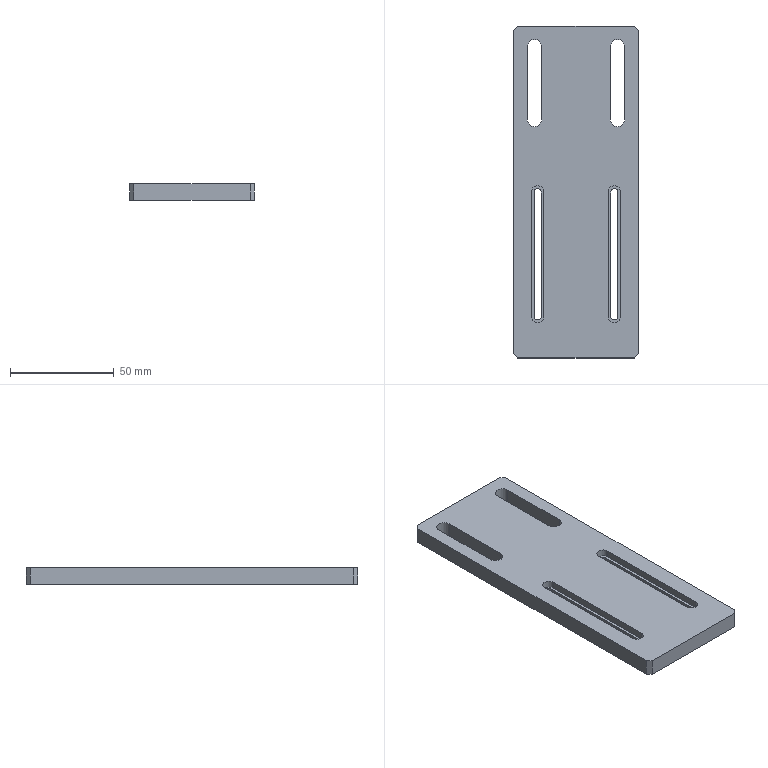Part | NX | 1 solid | 36 faces | box 60 x 160 x 8 mm | volume 67600 mm3 | plane 24 | cylinder 12 | commonest cylinder face diameters 3.4 x4 6 x4 7 x4
STEP:
#1=CARTESIAN_POINT('',(16.8,0.,4.6));
#2=VERTEX_POINT('',#1);
#3=CARTESIAN_POINT('',(20.2,0.,4.6));
#4=VERTEX_POINT('',#3);
#5=CARTESIAN_POINT('',(18.5,0.,4.6));
#6=DIRECTION('',(0.,0.,1.));
#7=DIRECTION('',(1.,0.,0.));
#8=AXIS2_PLACEMENT_3D('',#5,#6,#7);
#9=CIRCLE('',#8,1.7);
#10=EDGE_CURVE('',#2,#4,#9,.F.);
#11=ORIENTED_EDGE('',*,*,#10,.F.);
#12=CARTESIAN_POINT('',(16.8,0.,0.));
#13=VERTEX_POINT('',#12);
#14=CARTESIAN_POINT('',(16.8,0.,0.));
#15=DIRECTION('',(0.,0.,1.));
#16=VECTOR('',#15,1000.);
#17=LINE('',#14,#16);
#18=EDGE_CURVE('',#13,#2,#17,.T.);
#19=ORIENTED_EDGE('',*,*,#18,.F.);
#20=CARTESIAN_POINT('',(20.2,0.,0.));
#21=VERTEX_POINT('',#20);
#22=CARTESIAN_POINT('',(18.5,0.,0.));
#23=DIRECTION('',(0.,0.,1.));
#24=DIRECTION('',(1.,0.,0.));
#25=AXIS2_PLACEMENT_3D('',#22,#23,#24);
#26=CIRCLE('',#25,1.7);
#27=EDGE_CURVE('',#21,#13,#26,.T.);
#28=ORIENTED_EDGE('',*,*,#27,.F.);
#29=CARTESIAN_POINT('',(20.2,0.,0.));
#30=DIRECTION('',(0.,0.,1.));
#31=VECTOR('',#30,1000.);
#32=LINE('',#29,#31);
#33=EDGE_CURVE('',#21,#4,#32,.T.);
#34=ORIENTED_EDGE('',*,*,#33,.T.);
#35=EDGE_LOOP('',(#11,#19,#28,#34));
#36=FACE_BOUND('',#35,.T.);
#37=CARTESIAN_POINT('',(18.5,0.,0.));
#38=DIRECTION('',(0.,0.,1.));
#39=DIRECTION('',(1.,0.,0.));
#40=AXIS2_PLACEMENT_3D('',#37,#38,#39);
#41=CYLINDRICAL_SURFACE('',#40,1.7);
#42=ADVANCED_FACE('',(#36),#41,.F.);
#43=CARTESIAN_POINT('',(20.2,-60.,4.6));
#44=VERTEX_POINT('',#43);
#45=CARTESIAN_POINT('',(20.2,0.,4.6));
#46=DIRECTION('',(0.,-1.,0.));
#47=VECTOR('',#46,1000.);
#48=LINE('',#45,#47);
#49=EDGE_CURVE('',#4,#44,#48,.T.);
#50=ORIENTED_EDGE('',*,*,#49,.F.);
#51=ORIENTED_EDGE('',*,*,#33,.F.);
#52=CARTESIAN_POINT('',(20.2,-60.,0.));
#53=VERTEX_POINT('',#52);
#54=CARTESIAN_POINT('',(20.2,0.,0.));
#55=DIRECTION('',(0.,1.,0.));
#56=VECTOR('',#55,1000.);
#57=LINE('',#54,#56);
#58=EDGE_CURVE('',#53,#21,#57,.T.);
#59=ORIENTED_EDGE('',*,*,#58,.F.);
#60=CARTESIAN_POINT('',(20.2,-60.,0.));
#61=DIRECTION('',(0.,0.,1.));
#62=VECTOR('',#61,1000.);
#63=LINE('',#60,#62);
#64=EDGE_CURVE('',#53,#44,#63,.T.);
#65=ORIENTED_EDGE('',*,*,#64,.T.);
#66=EDGE_LOOP('',(#50,#51,#59,#65));
#67=FACE_BOUND('',#66,.T.);
#68=CARTESIAN_POINT('',(20.2,0.,0.));
#69=DIRECTION('',(1.,0.,0.));
#70=DIRECTION('',(0.,1.,0.));
#71=AXIS2_PLACEMENT_3D('',#68,#69,#70);
#72=PLANE('',#71);
#73=ADVANCED_FACE('',(#67),#72,.F.);
#74=CARTESIAN_POINT('',(16.8,-60.,4.6));
#75=VERTEX_POINT('',#74);
#76=CARTESIAN_POINT('',(18.5,-60.,4.6));
#77=DIRECTION('',(0.,0.,1.));
#78=DIRECTION('',(1.,0.,0.));
#79=AXIS2_PLACEMENT_3D('',#76,#77,#78);
#80=CIRCLE('',#79,1.7);
#81=EDGE_CURVE('',#44,#75,#80,.F.);
#82=ORIENTED_EDGE('',*,*,#81,.F.);
#83=ORIENTED_EDGE('',*,*,#64,.F.);
#84=CARTESIAN_POINT('',(16.8,-60.,0.));
#85=VERTEX_POINT('',#84);
#86=CARTESIAN_POINT('',(18.5,-60.,0.));
#87=DIRECTION('',(0.,0.,1.));
#88=DIRECTION('',(1.,0.,0.));
#89=AXIS2_PLACEMENT_3D('',#86,#87,#88);
#90=CIRCLE('',#89,1.7);
#91=EDGE_CURVE('',#85,#53,#90,.T.);
#92=ORIENTED_EDGE('',*,*,#91,.F.);
#93=CARTESIAN_POINT('',(16.8,-60.,0.));
#94=DIRECTION('',(0.,0.,1.));
#95=VECTOR('',#94,1000.);
#96=LINE('',#93,#95);
#97=EDGE_CURVE('',#85,#75,#96,.T.);
#98=ORIENTED_EDGE('',*,*,#97,.T.);
#99=EDGE_LOOP('',(#82,#83,#92,#98));
#100=FACE_BOUND('',#99,.T.);
#101=CARTESIAN_POINT('',(18.5,-60.,0.));
#102=DIRECTION('',(0.,0.,1.));
#103=DIRECTION('',(1.,0.,0.));
#104=AXIS2_PLACEMENT_3D('',#101,#102,#103);
#105=CYLINDRICAL_SURFACE('',#104,1.7);
#106=ADVANCED_FACE('',(#100),#105,.F.);
#107=CARTESIAN_POINT('',(16.8,0.,4.6));
#108=DIRECTION('',(0.,1.,0.));
#109=VECTOR('',#108,1000.);
#110=LINE('',#107,#109);
#111=EDGE_CURVE('',#75,#2,#110,.T.);
#112=ORIENTED_EDGE('',*,*,#111,.F.);
#113=ORIENTED_EDGE('',*,*,#97,.F.);
#114=CARTESIAN_POINT('',(16.8,0.,0.));
#115=DIRECTION('',(0.,-1.,0.));
#116=VECTOR('',#115,1000.);
#117=LINE('',#114,#116);
#118=EDGE_CURVE('',#13,#85,#117,.T.);
#119=ORIENTED_EDGE('',*,*,#118,.F.);
#120=ORIENTED_EDGE('',*,*,#18,.T.);
#121=EDGE_LOOP('',(#112,#113,#119,#120));
#122=FACE_BOUND('',#121,.T.);
#123=CARTESIAN_POINT('',(16.8,0.,0.));
#124=DIRECTION('',(-1.,0.,0.));
#125=DIRECTION('',(0.,-1.,0.));
#126=AXIS2_PLACEMENT_3D('',#123,#124,#125);
#127=PLANE('',#126);
#128=ADVANCED_FACE('',(#122),#127,.F.);
#129=CARTESIAN_POINT('',(-20.2,0.,4.6));
#130=VERTEX_POINT('',#129);
#131=CARTESIAN_POINT('',(-16.8,0.,4.6));
#132=VERTEX_POINT('',#131);
#133=CARTESIAN_POINT('',(-18.5,0.,4.6));
#134=DIRECTION('',(0.,0.,1.));
#135=DIRECTION('',(1.,0.,0.));
#136=AXIS2_PLACEMENT_3D('',#133,#134,#135);
#137=CIRCLE('',#136,1.7);
#138=EDGE_CURVE('',#130,#132,#137,.F.);
#139=ORIENTED_EDGE('',*,*,#138,.F.);
#140=CARTESIAN_POINT('',(-20.2,0.,0.));
#141=VERTEX_POINT('',#140);
#142=CARTESIAN_POINT('',(-20.2,0.,0.));
#143=DIRECTION('',(0.,0.,1.));
#144=VECTOR('',#143,1000.);
#145=LINE('',#142,#144);
#146=EDGE_CURVE('',#141,#130,#145,.T.);
#147=ORIENTED_EDGE('',*,*,#146,.F.);
#148=CARTESIAN_POINT('',(-16.8,0.,0.));
#149=VERTEX_POINT('',#148);
#150=CARTESIAN_POINT('',(-18.5,0.,0.));
#151=DIRECTION('',(0.,0.,1.));
#152=DIRECTION('',(1.,0.,0.));
#153=AXIS2_PLACEMENT_3D('',#150,#151,#152);
#154=CIRCLE('',#153,1.7);
#155=EDGE_CURVE('',#149,#141,#154,.T.);
#156=ORIENTED_EDGE('',*,*,#155,.F.);
#157=CARTESIAN_POINT('',(-16.8,0.,0.));
#158=DIRECTION('',(0.,0.,1.));
#159=VECTOR('',#158,1000.);
#160=LINE('',#157,#159);
#161=EDGE_CURVE('',#149,#132,#160,.T.);
#162=ORIENTED_EDGE('',*,*,#161,.T.);
#163=EDGE_LOOP('',(#139,#147,#156,#162));
#164=FACE_BOUND('',#163,.T.);
#165=CARTESIAN_POINT('',(-18.5,0.,0.));
#166=DIRECTION('',(0.,0.,1.));
#167=DIRECTION('',(1.,0.,0.));
#168=AXIS2_PLACEMENT_3D('',#165,#166,#167);
#169=CYLINDRICAL_SURFACE('',#168,1.7);
#170=ADVANCED_FACE('',(#164),#169,.F.);
#171=CARTESIAN_POINT('',(-16.8,-60.,4.6));
#172=VERTEX_POINT('',#171);
#173=CARTESIAN_POINT('',(-16.8,0.,4.6));
#174=DIRECTION('',(0.,-1.,0.));
#175=VECTOR('',#174,1000.);
#176=LINE('',#173,#175);
#177=EDGE_CURVE('',#132,#172,#176,.T.);
#178=ORIENTED_EDGE('',*,*,#177,.F.);
#179=ORIENTED_EDGE('',*,*,#161,.F.);
#180=CARTESIAN_POINT('',(-16.8,-60.,0.));
#181=VERTEX_POINT('',#180);
#182=CARTESIAN_POINT('',(-16.8,0.,0.));
#183=DIRECTION('',(0.,1.,0.));
#184=VECTOR('',#183,1000.);
#185=LINE('',#182,#184);
#186=EDGE_CURVE('',#181,#149,#185,.T.);
#187=ORIENTED_EDGE('',*,*,#186,.F.);
#188=CARTESIAN_POINT('',(-16.8,-60.,0.));
#189=DIRECTION('',(0.,0.,1.));
#190=VECTOR('',#189,1000.);
#191=LINE('',#188,#190);
#192=EDGE_CURVE('',#181,#172,#191,.T.);
#193=ORIENTED_EDGE('',*,*,#192,.T.);
#194=EDGE_LOOP('',(#178,#179,#187,#193));
#195=FACE_BOUND('',#194,.T.);
#196=CARTESIAN_POINT('',(-16.8,0.,0.));
#197=DIRECTION('',(1.,0.,0.));
#198=DIRECTION('',(0.,0.,-1.));
#199=AXIS2_PLACEMENT_3D('',#196,#197,#198);
#200=PLANE('',#199);
#201=ADVANCED_FACE('',(#195),#200,.F.);
#202=CARTESIAN_POINT('',(-20.2,-60.,4.6));
#203=VERTEX_POINT('',#202);
#204=CARTESIAN_POINT('',(-18.5,-60.,4.6));
#205=DIRECTION('',(0.,0.,1.));
#206=DIRECTION('',(1.,0.,0.));
#207=AXIS2_PLACEMENT_3D('',#204,#205,#206);
#208=CIRCLE('',#207,1.7);
#209=EDGE_CURVE('',#172,#203,#208,.F.);
#210=ORIENTED_EDGE('',*,*,#209,.F.);
#211=ORIENTED_EDGE('',*,*,#192,.F.);
#212=CARTESIAN_POINT('',(-20.2,-60.,0.));
#213=VERTEX_POINT('',#212);
#214=CARTESIAN_POINT('',(-18.5,-60.,0.));
#215=DIRECTION('',(0.,0.,1.));
#216=DIRECTION('',(1.,0.,0.));
#217=AXIS2_PLACEMENT_3D('',#214,#215,#216);
#218=CIRCLE('',#217,1.7);
#219=EDGE_CURVE('',#213,#181,#218,.T.);
#220=ORIENTED_EDGE('',*,*,#219,.F.);
#221=CARTESIAN_POINT('',(-20.2,-60.,0.));
#222=DIRECTION('',(0.,0.,1.));
#223=VECTOR('',#222,1000.);
#224=LINE('',#221,#223);
#225=EDGE_CURVE('',#213,#203,#224,.T.);
#226=ORIENTED_EDGE('',*,*,#225,.T.);
#227=EDGE_LOOP('',(#210,#211,#220,#226));
#228=FACE_BOUND('',#227,.T.);
#229=CARTESIAN_POINT('',(-18.5,-60.,0.));
#230=DIRECTION('',(0.,0.,1.));
#231=DIRECTION('',(1.,0.,0.));
#232=AXIS2_PLACEMENT_3D('',#229,#230,#231);
#233=CYLINDRICAL_SURFACE('',#232,1.7);
#234=ADVANCED_FACE('',(#228),#233,.F.);
#235=CARTESIAN_POINT('',(-20.2,0.,4.6));
#236=DIRECTION('',(0.,1.,0.));
#237=VECTOR('',#236,1000.);
#238=LINE('',#235,#237);
#239=EDGE_CURVE('',#203,#130,#238,.T.);
#240=ORIENTED_EDGE('',*,*,#239,.F.);
#241=ORIENTED_EDGE('',*,*,#225,.F.);
#242=CARTESIAN_POINT('',(-20.2,0.,0.));
#243=DIRECTION('',(0.,-1.,0.));
#244=VECTOR('',#243,1000.);
#245=LINE('',#242,#244);
#246=EDGE_CURVE('',#141,#213,#245,.T.);
#247=ORIENTED_EDGE('',*,*,#246,.F.);
#248=ORIENTED_EDGE('',*,*,#146,.T.);
#249=EDGE_LOOP('',(#240,#241,#247,#248));
#250=FACE_BOUND('',#249,.T.);
#251=CARTESIAN_POINT('',(-20.2,0.,0.));
#252=DIRECTION('',(-1.,0.,0.));
#253=DIRECTION('',(0.,0.,1.));
#254=AXIS2_PLACEMENT_3D('',#251,#252,#253);
#255=PLANE('',#254);
#256=ADVANCED_FACE('',(#250),#255,.F.);
#257=CARTESIAN_POINT('',(-30.,78.,0.));
#258=VERTEX_POINT('',#257);
#259=CARTESIAN_POINT('',(-30.,-78.,0.));
#260=VERTEX_POINT('',#259);
#261=CARTESIAN_POINT('',(-30.,-80.,0.));
#262=DIRECTION('',(0.,-1.,0.));
#263=VECTOR('',#262,1000.);
#264=LINE('',#261,#263);
#265=EDGE_CURVE('',#258,#260,#264,.T.);
#266=ORIENTED_EDGE('',*,*,#265,.T.);
#267=CARTESIAN_POINT('',(-30.,-78.,8.));
#268=VERTEX_POINT('',#267);
#269=CARTESIAN_POINT('',(-30.,-78.,8.));
#270=DIRECTION('',(0.,0.,1.));
#271=VECTOR('',#270,1000.);
#272=LINE('',#269,#271);
#273=EDGE_CURVE('',#260,#268,#272,.T.);
#274=ORIENTED_EDGE('',*,*,#273,.T.);
#275=CARTESIAN_POINT('',(-30.,78.,8.));
#276=VERTEX_POINT('',#275);
#277=CARTESIAN_POINT('',(-30.,-80.,8.));
#278=DIRECTION('',(0.,-1.,0.));
#279=VECTOR('',#278,1000.);
#280=LINE('',#277,#279);
#281=EDGE_CURVE('',#276,#268,#280,.T.);
#282=ORIENTED_EDGE('',*,*,#281,.F.);
#283=CARTESIAN_POINT('',(-30.,78.,8.));
#284=DIRECTION('',(0.,0.,-1.));
#285=VECTOR('',#284,1000.);
#286=LINE('',#283,#285);
#287=EDGE_CURVE('',#276,#258,#286,.T.);
#288=ORIENTED_EDGE('',*,*,#287,.T.);
#289=EDGE_LOOP('',(#266,#274,#282,#288));
#290=FACE_BOUND('',#289,.T.);
#291=CARTESIAN_POINT('',(-30.,-80.,8.));
#292=DIRECTION('',(1.,0.,0.));
#293=DIRECTION('',(0.,0.,-1.));
#294=AXIS2_PLACEMENT_3D('',#291,#292,#293);
#295=PLANE('',#294);
#296=ADVANCED_FACE('',(#290),#295,.F.);
#297=CARTESIAN_POINT('',(-28.,-80.,0.));
#298=VERTEX_POINT('',#297);
#299=CARTESIAN_POINT('',(28.,-80.,0.));
#300=VERTEX_POINT('',#299);
#301=CARTESIAN_POINT('',(30.,-80.,0.));
#302=DIRECTION('',(1.,0.,0.));
#303=VECTOR('',#302,1000.);
#304=LINE('',#301,#303);
#305=EDGE_CURVE('',#298,#300,#304,.T.);
#306=ORIENTED_EDGE('',*,*,#305,.T.);
#307=CARTESIAN_POINT('',(28.,-80.,8.));
#308=VERTEX_POINT('',#307);
#309=CARTESIAN_POINT('',(28.,-80.,8.));
#310=DIRECTION('',(0.,0.,1.));
#311=VECTOR('',#310,1000.);
#312=LINE('',#309,#311);
#313=EDGE_CURVE('',#300,#308,#312,.T.);
#314=ORIENTED_EDGE('',*,*,#313,.T.);
#315=CARTESIAN_POINT('',(-28.,-80.,8.));
#316=VERTEX_POINT('',#315);
#317=CARTESIAN_POINT('',(30.,-80.,8.));
#318=DIRECTION('',(1.,0.,0.));
#319=VECTOR('',#318,1000.);
#320=LINE('',#317,#319);
#321=EDGE_CURVE('',#316,#308,#320,.T.);
#322=ORIENTED_EDGE('',*,*,#321,.F.);
#323=CARTESIAN_POINT('',(-28.,-80.,8.));
#324=DIRECTION('',(0.,0.,-1.));
#325=VECTOR('',#324,1000.);
#326=LINE('',#323,#325);
#327=EDGE_CURVE('',#316,#298,#326,.T.);
#328=ORIENTED_EDGE('',*,*,#327,.T.);
#329=EDGE_LOOP('',(#306,#314,#322,#328));
#330=FACE_BOUND('',#329,.T.);
#331=CARTESIAN_POINT('',(30.,-80.,8.));
#332=DIRECTION('',(0.,1.,0.));
#333=DIRECTION('',(-1.,0.,0.));
#334=AXIS2_PLACEMENT_3D('',#331,#332,#333);
#335=PLANE('',#334);
#336=ADVANCED_FACE('',(#330),#335,.F.);
#337=CARTESIAN_POINT('',(30.,-78.,8.));
#338=VERTEX_POINT('',#337);
#339=CARTESIAN_POINT('',(30.,78.,8.));
#340=VERTEX_POINT('',#339);
#341=CARTESIAN_POINT('',(30.,-80.,8.));
#342=DIRECTION('',(0.,1.,0.));
#343=VECTOR('',#342,1000.);
#344=LINE('',#341,#343);
#345=EDGE_CURVE('',#338,#340,#344,.T.);
#346=ORIENTED_EDGE('',*,*,#345,.F.);
#347=CARTESIAN_POINT('',(30.,-78.,0.));
#348=VERTEX_POINT('',#347);
#349=CARTESIAN_POINT('',(30.,-78.,8.));
#350=DIRECTION('',(0.,0.,-1.));
#351=VECTOR('',#350,1000.);
#352=LINE('',#349,#351);
#353=EDGE_CURVE('',#338,#348,#352,.T.);
#354=ORIENTED_EDGE('',*,*,#353,.T.);
#355=CARTESIAN_POINT('',(30.,78.,0.));
#356=VERTEX_POINT('',#355);
#357=CARTESIAN_POINT('',(30.,-80.,0.));
#358=DIRECTION('',(0.,1.,0.));
#359=VECTOR('',#358,1000.);
#360=LINE('',#357,#359);
#361=EDGE_CURVE('',#348,#356,#360,.T.);
#362=ORIENTED_EDGE('',*,*,#361,.T.);
#363=CARTESIAN_POINT('',(30.,78.,8.));
#364=DIRECTION('',(0.,0.,1.));
#365=VECTOR('',#364,1000.);
#366=LINE('',#363,#365);
#367=EDGE_CURVE('',#356,#340,#366,.T.);
#368=ORIENTED_EDGE('',*,*,#367,.T.);
#369=EDGE_LOOP('',(#346,#354,#362,#368));
#370=FACE_BOUND('',#369,.T.);
#371=CARTESIAN_POINT('',(30.,-80.,8.));
#372=DIRECTION('',(-1.,0.,0.));
#373=DIRECTION('',(0.,0.,1.));
#374=AXIS2_PLACEMENT_3D('',#371,#372,#373);
#375=PLANE('',#374);
#376=ADVANCED_FACE('',(#370),#375,.F.);
#377=CARTESIAN_POINT('',(28.,80.,0.));
#378=VERTEX_POINT('',#377);
#379=CARTESIAN_POINT('',(-28.,80.,0.));
#380=VERTEX_POINT('',#379);
#381=CARTESIAN_POINT('',(30.,80.,0.));
#382=DIRECTION('',(-1.,0.,0.));
#383=VECTOR('',#382,1000.);
#384=LINE('',#381,#383);
#385=EDGE_CURVE('',#378,#380,#384,.T.);
#386=ORIENTED_EDGE('',*,*,#385,.T.);
#387=CARTESIAN_POINT('',(-28.,80.,8.));
#388=VERTEX_POINT('',#387);
#389=CARTESIAN_POINT('',(-28.,80.,8.));
#390=DIRECTION('',(0.,0.,1.));
#391=VECTOR('',#390,1000.);
#392=LINE('',#389,#391);
#393=EDGE_CURVE('',#380,#388,#392,.T.);
#394=ORIENTED_EDGE('',*,*,#393,.T.);
#395=CARTESIAN_POINT('',(28.,80.,8.));
#396=VERTEX_POINT('',#395);
#397=CARTESIAN_POINT('',(30.,80.,8.));
#398=DIRECTION('',(-1.,0.,0.));
#399=VECTOR('',#398,1000.);
#400=LINE('',#397,#399);
#401=EDGE_CURVE('',#396,#388,#400,.T.);
#402=ORIENTED_EDGE('',*,*,#401,.F.);
#403=CARTESIAN_POINT('',(28.,80.,8.));
#404=DIRECTION('',(0.,0.,-1.));
#405=VECTOR('',#404,1000.);
#406=LINE('',#403,#405);
#407=EDGE_CURVE('',#396,#378,#406,.T.);
#408=ORIENTED_EDGE('',*,*,#407,.T.);
#409=EDGE_LOOP('',(#386,#394,#402,#408));
#410=FACE_BOUND('',#409,.T.);
#411=CARTESIAN_POINT('',(30.,80.,8.));
#412=DIRECTION('',(0.,-1.,0.));
#413=DIRECTION('',(0.,0.,-1.));
#414=AXIS2_PLACEMENT_3D('',#411,#412,#413);
#415=PLANE('',#414);
#416=ADVANCED_FACE('',(#410),#415,.F.);
#417=CARTESIAN_POINT('',(15.5,-60.,8.));
#418=VERTEX_POINT('',#417);
#419=CARTESIAN_POINT('',(21.5,-60.,8.));
#420=VERTEX_POINT('',#419);
#421=CARTESIAN_POINT('',(18.5,-60.,8.));
#422=DIRECTION('',(0.,0.,1.));
#423=DIRECTION('',(1.,0.,0.));
#424=AXIS2_PLACEMENT_3D('',#421,#422,#423);
#425=CIRCLE('',#424,3.);
#426=EDGE_CURVE('',#418,#420,#425,.T.);
#427=ORIENTED_EDGE('',*,*,#426,.F.);
#428=CARTESIAN_POINT('',(15.5,0.,8.));
#429=VERTEX_POINT('',#428);
#430=CARTESIAN_POINT('',(15.5,-60.,8.));
#431=DIRECTION('',(0.,-1.,0.));
#432=VECTOR('',#431,1000.);
#433=LINE('',#430,#432);
#434=EDGE_CURVE('',#429,#418,#433,.T.);
#435=ORIENTED_EDGE('',*,*,#434,.F.);
#436=CARTESIAN_POINT('',(21.5,0.,8.));
#437=VERTEX_POINT('',#436);
#438=CARTESIAN_POINT('',(18.5,0.,8.));
#439=DIRECTION('',(0.,0.,1.));
#440=DIRECTION('',(1.,0.,0.));
#441=AXIS2_PLACEMENT_3D('',#438,#439,#440);
#442=CIRCLE('',#441,3.);
#443=EDGE_CURVE('',#437,#429,#442,.T.);
#444=ORIENTED_EDGE('',*,*,#443,.F.);
#445=CARTESIAN_POINT('',(21.5,-60.,8.));
#446=DIRECTION('',(0.,1.,0.));
#447=VECTOR('',#446,1000.);
#448=LINE('',#445,#447);
#449=EDGE_CURVE('',#420,#437,#448,.T.);
#450=ORIENTED_EDGE('',*,*,#449,.F.);
#451=EDGE_LOOP('',(#427,#435,#444,#450));
#452=FACE_BOUND('',#451,.T.);
#453=CARTESIAN_POINT('',(-15.5,0.,8.));
#454=VERTEX_POINT('',#453);
#455=CARTESIAN_POINT('',(-21.5,0.,8.));
#456=VERTEX_POINT('',#455);
#457=CARTESIAN_POINT('',(-18.5,0.,8.));
#458=DIRECTION('',(0.,0.,1.));
#459=DIRECTION('',(1.,0.,0.));
#460=AXIS2_PLACEMENT_3D('',#457,#458,#459);
#461=CIRCLE('',#460,3.);
#462=EDGE_CURVE('',#454,#456,#461,.T.);
#463=ORIENTED_EDGE('',*,*,#462,.F.);
#464=CARTESIAN_POINT('',(-15.5,-60.,8.));
#465=VERTEX_POINT('',#464);
#466=CARTESIAN_POINT('',(-15.5,0.,8.));
#467=DIRECTION('',(0.,1.,0.));
#468=VECTOR('',#467,1000.);
#469=LINE('',#466,#468);
#470=EDGE_CURVE('',#465,#454,#469,.T.);
#471=ORIENTED_EDGE('',*,*,#470,.F.);
#472=CARTESIAN_POINT('',(-21.5,-60.,8.));
#473=VERTEX_POINT('',#472);
#474=CARTESIAN_POINT('',(-18.5,-60.,8.));
#475=DIRECTION('',(0.,0.,1.));
#476=DIRECTION('',(1.,0.,0.));
#477=AXIS2_PLACEMENT_3D('',#474,#475,#476);
#478=CIRCLE('',#477,3.);
#479=EDGE_CURVE('',#473,#465,#478,.T.);
#480=ORIENTED_EDGE('',*,*,#479,.F.);
#481=CARTESIAN_POINT('',(-21.5,0.,8.));
#482=DIRECTION('',(0.,-1.,0.));
#483=VECTOR('',#482,1000.);
#484=LINE('',#481,#483);
#485=EDGE_CURVE('',#456,#473,#484,.T.);
#486=ORIENTED_EDGE('',*,*,#485,.F.);
#487=EDGE_LOOP('',(#463,#471,#480,#486));
#488=FACE_BOUND('',#487,.T.);
#489=CARTESIAN_POINT('',(23.5,70.,8.));
#490=VERTEX_POINT('',#489);
#491=CARTESIAN_POINT('',(16.5,70.,8.));
#492=VERTEX_POINT('',#491);
#493=CARTESIAN_POINT('',(20.,70.,8.));
#494=DIRECTION('',(0.,0.,1.));
#495=DIRECTION('',(1.,0.,0.));
#496=AXIS2_PLACEMENT_3D('',#493,#494,#495);
#497=CIRCLE('',#496,3.5);
#498=EDGE_CURVE('',#490,#492,#497,.T.);
#499=ORIENTED_EDGE('',*,*,#498,.F.);
#500=CARTESIAN_POINT('',(23.5,35.,8.));
#501=VERTEX_POINT('',#500);
#502=CARTESIAN_POINT('',(23.5,70.,8.));
#503=DIRECTION('',(0.,1.,0.));
#504=VECTOR('',#503,1000.);
#505=LINE('',#502,#504);
#506=EDGE_CURVE('',#501,#490,#505,.T.);
#507=ORIENTED_EDGE('',*,*,#506,.F.);
#508=CARTESIAN_POINT('',(16.5,35.,8.));
#509=VERTEX_POINT('',#508);
#510=CARTESIAN_POINT('',(20.,35.,8.));
#511=DIRECTION('',(0.,0.,1.));
#512=DIRECTION('',(1.,0.,0.));
#513=AXIS2_PLACEMENT_3D('',#510,#511,#512);
#514=CIRCLE('',#513,3.5);
#515=EDGE_CURVE('',#509,#501,#514,.T.);
#516=ORIENTED_EDGE('',*,*,#515,.F.);
#517=CARTESIAN_POINT('',(16.5,70.,8.));
#518=DIRECTION('',(0.,-1.,0.));
#519=VECTOR('',#518,1000.);
#520=LINE('',#517,#519);
#521=EDGE_CURVE('',#492,#509,#520,.T.);
#522=ORIENTED_EDGE('',*,*,#521,.F.);
#523=EDGE_LOOP('',(#499,#507,#516,#522));
#524=FACE_BOUND('',#523,.T.);
#525=CARTESIAN_POINT('',(-16.5,70.,8.));
#526=VERTEX_POINT('',#525);
#527=CARTESIAN_POINT('',(-23.5,70.,8.));
#528=VERTEX_POINT('',#527);
#529=CARTESIAN_POINT('',(-20.,70.,8.));
#530=DIRECTION('',(0.,0.,1.));
#531=DIRECTION('',(1.,0.,0.));
#532=AXIS2_PLACEMENT_3D('',#529,#530,#531);
#533=CIRCLE('',#532,3.5);
#534=EDGE_CURVE('',#526,#528,#533,.T.);
#535=ORIENTED_EDGE('',*,*,#534,.F.);
#536=CARTESIAN_POINT('',(-16.5,35.,8.));
#537=VERTEX_POINT('',#536);
#538=CARTESIAN_POINT('',(-16.5,70.,8.));
#539=DIRECTION('',(0.,1.,0.));
#540=VECTOR('',#539,1000.);
#541=LINE('',#538,#540);
#542=EDGE_CURVE('',#537,#526,#541,.T.);
#543=ORIENTED_EDGE('',*,*,#542,.F.);
#544=CARTESIAN_POINT('',(-23.5,35.,8.));
#545=VERTEX_POINT('',#544);
#546=CARTESIAN_POINT('',(-20.,35.,8.));
#547=DIRECTION('',(0.,0.,1.));
#548=DIRECTION('',(1.,0.,0.));
#549=AXIS2_PLACEMENT_3D('',#546,#547,#548);
#550=CIRCLE('',#549,3.5);
#551=EDGE_CURVE('',#545,#537,#550,.T.);
#552=ORIENTED_EDGE('',*,*,#551,.F.);
#553=CARTESIAN_POINT('',(-23.5,70.,8.));
#554=DIRECTION('',(0.,-1.,0.));
#555=VECTOR('',#554,1000.);
#556=LINE('',#553,#555);
#557=EDGE_CURVE('',#528,#545,#556,.T.);
#558=ORIENTED_EDGE('',*,*,#557,.F.);
#559=EDGE_LOOP('',(#535,#543,#552,#558));
#560=FACE_BOUND('',#559,.T.);
#561=ORIENTED_EDGE('',*,*,#321,.T.);
#562=CARTESIAN_POINT('',(54.,-54.,8.));
#563=DIRECTION('',(-0.7071,-0.7071,0.));
#564=VECTOR('',#563,1000.);
#565=LINE('',#562,#564);
#566=EDGE_CURVE('',#308,#338,#565,.F.);
#567=ORIENTED_EDGE('',*,*,#566,.T.);
#568=ORIENTED_EDGE('',*,*,#345,.T.);
#569=CARTESIAN_POINT('',(54.,54.,8.));
#570=DIRECTION('',(0.7071,-0.7071,0.));
#571=VECTOR('',#570,1000.);
#572=LINE('',#569,#571);
#573=EDGE_CURVE('',#340,#396,#572,.F.);
#574=ORIENTED_EDGE('',*,*,#573,.T.);
#575=ORIENTED_EDGE('',*,*,#401,.T.);
#576=CARTESIAN_POINT('',(-54.,54.,8.));
#577=DIRECTION('',(0.7071,0.7071,0.));
#578=VECTOR('',#577,1000.);
#579=LINE('',#576,#578);
#580=EDGE_CURVE('',#388,#276,#579,.F.);
#581=ORIENTED_EDGE('',*,*,#580,.T.);
#582=ORIENTED_EDGE('',*,*,#281,.T.);
#583=CARTESIAN_POINT('',(-54.,-54.,8.));
#584=DIRECTION('',(-0.7071,0.7071,0.));
#585=VECTOR('',#584,1000.);
#586=LINE('',#583,#585);
#587=EDGE_CURVE('',#268,#316,#586,.F.);
#588=ORIENTED_EDGE('',*,*,#587,.T.);
#589=EDGE_LOOP('',(#561,#567,#568,#574,#575,#581,#582,#588));
#590=FACE_BOUND('',#589,.T.);
#591=CARTESIAN_POINT('',(0.,0.,8.));
#592=DIRECTION('',(0.,0.,1.));
#593=DIRECTION('',(1.,0.,0.));
#594=AXIS2_PLACEMENT_3D('',#591,#592,#593);
#595=PLANE('',#594);
#596=ADVANCED_FACE('',(#452,#488,#524,#560,#590),#595,.T.);
#597=ORIENTED_EDGE('',*,*,#58,.T.);
#598=ORIENTED_EDGE('',*,*,#27,.T.);
#599=ORIENTED_EDGE('',*,*,#118,.T.);
#600=ORIENTED_EDGE('',*,*,#91,.T.);
#601=EDGE_LOOP('',(#597,#598,#599,#600));
#602=FACE_BOUND('',#601,.T.);
#603=ORIENTED_EDGE('',*,*,#186,.T.);
#604=ORIENTED_EDGE('',*,*,#155,.T.);
#605=ORIENTED_EDGE('',*,*,#246,.T.);
#606=ORIENTED_EDGE('',*,*,#219,.T.);
#607=EDGE_LOOP('',(#603,#604,#605,#606));
#608=FACE_BOUND('',#607,.T.);
#609=CARTESIAN_POINT('',(23.5,35.,0.));
#610=VERTEX_POINT('',#609);
#611=CARTESIAN_POINT('',(23.5,70.,0.));
#612=VERTEX_POINT('',#611);
#613=CARTESIAN_POINT('',(23.5,70.,0.));
#614=DIRECTION('',(0.,1.,0.));
#615=VECTOR('',#614,1000.);
#616=LINE('',#613,#615);
#617=EDGE_CURVE('',#610,#612,#616,.T.);
#618=ORIENTED_EDGE('',*,*,#617,.T.);
#619=CARTESIAN_POINT('',(16.5,70.,0.));
#620=VERTEX_POINT('',#619);
#621=CARTESIAN_POINT('',(20.,70.,0.));
#622=DIRECTION('',(0.,0.,1.));
#623=DIRECTION('',(1.,0.,0.));
#624=AXIS2_PLACEMENT_3D('',#621,#622,#623);
#625=CIRCLE('',#624,3.5);
#626=EDGE_CURVE('',#612,#620,#625,.T.);
#627=ORIENTED_EDGE('',*,*,#626,.T.);
#628=CARTESIAN_POINT('',(16.5,35.,0.));
#629=VERTEX_POINT('',#628);
#630=CARTESIAN_POINT('',(16.5,70.,0.));
#631=DIRECTION('',(0.,-1.,0.));
#632=VECTOR('',#631,1000.);
#633=LINE('',#630,#632);
#634=EDGE_CURVE('',#620,#629,#633,.T.);
#635=ORIENTED_EDGE('',*,*,#634,.T.);
#636=CARTESIAN_POINT('',(20.,35.,0.));
#637=DIRECTION('',(0.,0.,1.));
#638=DIRECTION('',(1.,0.,0.));
#639=AXIS2_PLACEMENT_3D('',#636,#637,#638);
#640=CIRCLE('',#639,3.5);
#641=EDGE_CURVE('',#629,#610,#640,.T.);
#642=ORIENTED_EDGE('',*,*,#641,.T.);
#643=EDGE_LOOP('',(#618,#627,#635,#642));
#644=FACE_BOUND('',#643,.T.);
#645=CARTESIAN_POINT('',(-16.5,35.,0.));
#646=VERTEX_POINT('',#645);
#647=CARTESIAN_POINT('',(-16.5,70.,0.));
#648=VERTEX_POINT('',#647);
#649=CARTESIAN_POINT('',(-16.5,70.,0.));
#650=DIRECTION('',(0.,1.,0.));
#651=VECTOR('',#650,1000.);
#652=LINE('',#649,#651);
#653=EDGE_CURVE('',#646,#648,#652,.T.);
#654=ORIENTED_EDGE('',*,*,#653,.T.);
#655=CARTESIAN_POINT('',(-23.5,70.,0.));
#656=VERTEX_POINT('',#655);
#657=CARTESIAN_POINT('',(-20.,70.,0.));
#658=DIRECTION('',(0.,0.,1.));
#659=DIRECTION('',(1.,0.,0.));
#660=AXIS2_PLACEMENT_3D('',#657,#658,#659);
#661=CIRCLE('',#660,3.5);
#662=EDGE_CURVE('',#648,#656,#661,.T.);
#663=ORIENTED_EDGE('',*,*,#662,.T.);
#664=CARTESIAN_POINT('',(-23.5,35.,0.));
#665=VERTEX_POINT('',#664);
#666=CARTESIAN_POINT('',(-23.5,70.,0.));
#667=DIRECTION('',(0.,-1.,0.));
#668=VECTOR('',#667,1000.);
#669=LINE('',#666,#668);
#670=EDGE_CURVE('',#656,#665,#669,.T.);
#671=ORIENTED_EDGE('',*,*,#670,.T.);
#672=CARTESIAN_POINT('',(-20.,35.,0.));
#673=DIRECTION('',(0.,0.,1.));
#674=DIRECTION('',(1.,0.,0.));
#675=AXIS2_PLACEMENT_3D('',#672,#673,#674);
#676=CIRCLE('',#675,3.5);
#677=EDGE_CURVE('',#665,#646,#676,.T.);
#678=ORIENTED_EDGE('',*,*,#677,.T.);
#679=EDGE_LOOP('',(#654,#663,#671,#678));
#680=FACE_BOUND('',#679,.T.);
#681=ORIENTED_EDGE('',*,*,#361,.F.);
#682=CARTESIAN_POINT('',(30.,-78.,0.));
#683=DIRECTION('',(0.7071,0.7071,0.));
#684=VECTOR('',#683,1000.);
#685=LINE('',#682,#684);
#686=EDGE_CURVE('',#348,#300,#685,.F.);
#687=ORIENTED_EDGE('',*,*,#686,.T.);
#688=ORIENTED_EDGE('',*,*,#305,.F.);
#689=CARTESIAN_POINT('',(-28.,-80.,0.));
#690=DIRECTION('',(0.7071,-0.7071,0.));
#691=VECTOR('',#690,1000.);
#692=LINE('',#689,#691);
#693=EDGE_CURVE('',#298,#260,#692,.F.);
#694=ORIENTED_EDGE('',*,*,#693,.T.);
#695=ORIENTED_EDGE('',*,*,#265,.F.);
#696=CARTESIAN_POINT('',(-30.,78.,0.));
#697=DIRECTION('',(-0.7071,-0.7071,0.));
#698=VECTOR('',#697,1000.);
#699=LINE('',#696,#698);
#700=EDGE_CURVE('',#258,#380,#699,.F.);
#701=ORIENTED_EDGE('',*,*,#700,.T.);
#702=ORIENTED_EDGE('',*,*,#385,.F.);
#703=CARTESIAN_POINT('',(28.,80.,0.));
#704=DIRECTION('',(-0.7071,0.7071,0.));
#705=VECTOR('',#704,1000.);
#706=LINE('',#703,#705);
#707=EDGE_CURVE('',#378,#356,#706,.F.);
#708=ORIENTED_EDGE('',*,*,#707,.T.);
#709=EDGE_LOOP('',(#681,#687,#688,#694,#695,#701,#702,#708));
#710=FACE_BOUND('',#709,.T.);
#711=CARTESIAN_POINT('',(0.,0.,0.));
#712=DIRECTION('',(0.,0.,1.));
#713=DIRECTION('',(1.,0.,0.));
#714=AXIS2_PLACEMENT_3D('',#711,#712,#713);
#715=PLANE('',#714);
#716=ADVANCED_FACE('',(#602,#608,#644,#680,#710),#715,.F.);
#717=ORIENTED_EDGE('',*,*,#566,.F.);
#718=ORIENTED_EDGE('',*,*,#313,.F.);
#719=ORIENTED_EDGE('',*,*,#686,.F.);
#720=ORIENTED_EDGE('',*,*,#353,.F.);
#721=EDGE_LOOP('',(#717,#718,#719,#720));
#722=FACE_BOUND('',#721,.T.);
#723=CARTESIAN_POINT('',(30.,-78.,8.));
#724=DIRECTION('',(-0.7071,0.7071,0.));
#725=DIRECTION('',(0.,0.,-1.));
#726=AXIS2_PLACEMENT_3D('',#723,#724,#725);
#727=PLANE('',#726);
#728=ADVANCED_FACE('',(#722),#727,.F.);
#729=ORIENTED_EDGE('',*,*,#587,.F.);
#730=ORIENTED_EDGE('',*,*,#273,.F.);
#731=ORIENTED_EDGE('',*,*,#693,.F.);
#732=ORIENTED_EDGE('',*,*,#327,.F.);
#733=EDGE_LOOP('',(#729,#730,#731,#732));
#734=FACE_BOUND('',#733,.T.);
#735=CARTESIAN_POINT('',(-28.,-80.,8.));
#736=DIRECTION('',(0.7071,0.7071,0.));
#737=DIRECTION('',(0.,0.,-1.));
#738=AXIS2_PLACEMENT_3D('',#735,#736,#737);
#739=PLANE('',#738);
#740=ADVANCED_FACE('',(#734),#739,.F.);
#741=ORIENTED_EDGE('',*,*,#580,.F.);
#742=ORIENTED_EDGE('',*,*,#393,.F.);
#743=ORIENTED_EDGE('',*,*,#700,.F.);
#744=ORIENTED_EDGE('',*,*,#287,.F.);
#745=EDGE_LOOP('',(#741,#742,#743,#744));
#746=FACE_BOUND('',#745,.T.);
#747=CARTESIAN_POINT('',(-30.,78.,8.));
#748=DIRECTION('',(0.7071,-0.7071,0.));
#749=DIRECTION('',(0.,0.,-1.));
#750=AXIS2_PLACEMENT_3D('',#747,#748,#749);
#751=PLANE('',#750);
#752=ADVANCED_FACE('',(#746),#751,.F.);
#753=ORIENTED_EDGE('',*,*,#573,.F.);
#754=ORIENTED_EDGE('',*,*,#367,.F.);
#755=ORIENTED_EDGE('',*,*,#707,.F.);
#756=ORIENTED_EDGE('',*,*,#407,.F.);
#757=EDGE_LOOP('',(#753,#754,#755,#756));
#758=FACE_BOUND('',#757,.T.);
#759=CARTESIAN_POINT('',(28.,80.,8.));
#760=DIRECTION('',(-0.7071,-0.7071,0.));
#761=DIRECTION('',(0.,0.,-1.));
#762=AXIS2_PLACEMENT_3D('',#759,#760,#761);
#763=PLANE('',#762);
#764=ADVANCED_FACE('',(#758),#763,.F.);
#765=ORIENTED_EDGE('',*,*,#534,.T.);
#766=CARTESIAN_POINT('',(-23.5,70.,0.));
#767=DIRECTION('',(0.,0.,1.));
#768=VECTOR('',#767,1000.);
#769=LINE('',#766,#768);
#770=EDGE_CURVE('',#656,#528,#769,.T.);
#771=ORIENTED_EDGE('',*,*,#770,.F.);
#772=ORIENTED_EDGE('',*,*,#662,.F.);
#773=CARTESIAN_POINT('',(-16.5,70.,0.));
#774=DIRECTION('',(0.,0.,1.));
#775=VECTOR('',#774,1000.);
#776=LINE('',#773,#775);
#777=EDGE_CURVE('',#648,#526,#776,.T.);
#778=ORIENTED_EDGE('',*,*,#777,.T.);
#779=EDGE_LOOP('',(#765,#771,#772,#778));
#780=FACE_BOUND('',#779,.T.);
#781=CARTESIAN_POINT('',(-20.,70.,0.));
#782=DIRECTION('',(0.,0.,1.));
#783=DIRECTION('',(1.,0.,0.));
#784=AXIS2_PLACEMENT_3D('',#781,#782,#783);
#785=CYLINDRICAL_SURFACE('',#784,3.5);
#786=ADVANCED_FACE('',(#780),#785,.F.);
#787=ORIENTED_EDGE('',*,*,#542,.T.);
#788=ORIENTED_EDGE('',*,*,#777,.F.);
#789=ORIENTED_EDGE('',*,*,#653,.F.);
#790=CARTESIAN_POINT('',(-16.5,35.,0.));
#791=DIRECTION('',(0.,0.,1.));
#792=VECTOR('',#791,1000.);
#793=LINE('',#790,#792);
#794=EDGE_CURVE('',#646,#537,#793,.T.);
#795=ORIENTED_EDGE('',*,*,#794,.T.);
#796=EDGE_LOOP('',(#787,#788,#789,#795));
#797=FACE_BOUND('',#796,.T.);
#798=CARTESIAN_POINT('',(-16.5,70.,0.));
#799=DIRECTION('',(1.,0.,0.));
#800=DIRECTION('',(0.,1.,0.));
#801=AXIS2_PLACEMENT_3D('',#798,#799,#800);
#802=PLANE('',#801);
#803=ADVANCED_FACE('',(#797),#802,.F.);
#804=ORIENTED_EDGE('',*,*,#551,.T.);
#805=ORIENTED_EDGE('',*,*,#794,.F.);
#806=ORIENTED_EDGE('',*,*,#677,.F.);
#807=CARTESIAN_POINT('',(-23.5,35.,0.));
#808=DIRECTION('',(0.,0.,1.));
#809=VECTOR('',#808,1000.);
#810=LINE('',#807,#809);
#811=EDGE_CURVE('',#665,#545,#810,.T.);
#812=ORIENTED_EDGE('',*,*,#811,.T.);
#813=EDGE_LOOP('',(#804,#805,#806,#812));
#814=FACE_BOUND('',#813,.T.);
#815=CARTESIAN_POINT('',(-20.,35.,0.));
#816=DIRECTION('',(0.,0.,1.));
#817=DIRECTION('',(1.,0.,0.));
#818=AXIS2_PLACEMENT_3D('',#815,#816,#817);
#819=CYLINDRICAL_SURFACE('',#818,3.5);
#820=ADVANCED_FACE('',(#814),#819,.F.);
#821=ORIENTED_EDGE('',*,*,#557,.T.);
#822=ORIENTED_EDGE('',*,*,#811,.F.);
#823=ORIENTED_EDGE('',*,*,#670,.F.);
#824=ORIENTED_EDGE('',*,*,#770,.T.);
#825=EDGE_LOOP('',(#821,#822,#823,#824));
#826=FACE_BOUND('',#825,.T.);
#827=CARTESIAN_POINT('',(-23.5,70.,0.));
#828=DIRECTION('',(-1.,0.,0.));
#829=DIRECTION('',(0.,-1.,0.));
#830=AXIS2_PLACEMENT_3D('',#827,#828,#829);
#831=PLANE('',#830);
#832=ADVANCED_FACE('',(#826),#831,.F.);
#833=ORIENTED_EDGE('',*,*,#498,.T.);
#834=CARTESIAN_POINT('',(16.5,70.,0.));
#835=DIRECTION('',(0.,0.,1.));
#836=VECTOR('',#835,1000.);
#837=LINE('',#834,#836);
#838=EDGE_CURVE('',#620,#492,#837,.T.);
#839=ORIENTED_EDGE('',*,*,#838,.F.);
#840=ORIENTED_EDGE('',*,*,#626,.F.);
#841=CARTESIAN_POINT('',(23.5,70.,0.));
#842=DIRECTION('',(0.,0.,1.));
#843=VECTOR('',#842,1000.);
#844=LINE('',#841,#843);
#845=EDGE_CURVE('',#612,#490,#844,.T.);
#846=ORIENTED_EDGE('',*,*,#845,.T.);
#847=EDGE_LOOP('',(#833,#839,#840,#846));
#848=FACE_BOUND('',#847,.T.);
#849=CARTESIAN_POINT('',(20.,70.,0.));
#850=DIRECTION('',(0.,0.,1.));
#851=DIRECTION('',(1.,0.,0.));
#852=AXIS2_PLACEMENT_3D('',#849,#850,#851);
#853=CYLINDRICAL_SURFACE('',#852,3.5);
#854=ADVANCED_FACE('',(#848),#853,.F.);
#855=ORIENTED_EDGE('',*,*,#506,.T.);
#856=ORIENTED_EDGE('',*,*,#845,.F.);
#857=ORIENTED_EDGE('',*,*,#617,.F.);
#858=CARTESIAN_POINT('',(23.5,35.,0.));
#859=DIRECTION('',(0.,0.,1.));
#860=VECTOR('',#859,1000.);
#861=LINE('',#858,#860);
#862=EDGE_CURVE('',#610,#501,#861,.T.);
#863=ORIENTED_EDGE('',*,*,#862,.T.);
#864=EDGE_LOOP('',(#855,#856,#857,#863));
#865=FACE_BOUND('',#864,.T.);
#866=CARTESIAN_POINT('',(23.5,70.,0.));
#867=DIRECTION('',(1.,0.,0.));
#868=DIRECTION('',(0.,1.,0.));
#869=AXIS2_PLACEMENT_3D('',#866,#867,#868);
#870=PLANE('',#869);
#871=ADVANCED_FACE('',(#865),#870,.F.);
#872=ORIENTED_EDGE('',*,*,#515,.T.);
#873=ORIENTED_EDGE('',*,*,#862,.F.);
#874=ORIENTED_EDGE('',*,*,#641,.F.);
#875=CARTESIAN_POINT('',(16.5,35.,0.));
#876=DIRECTION('',(0.,0.,1.));
#877=VECTOR('',#876,1000.);
#878=LINE('',#875,#877);
#879=EDGE_CURVE('',#629,#509,#878,.T.);
#880=ORIENTED_EDGE('',*,*,#879,.T.);
#881=EDGE_LOOP('',(#872,#873,#874,#880));
#882=FACE_BOUND('',#881,.T.);
#883=CARTESIAN_POINT('',(20.,35.,0.));
#884=DIRECTION('',(0.,0.,1.));
#885=DIRECTION('',(1.,0.,0.));
#886=AXIS2_PLACEMENT_3D('',#883,#884,#885);
#887=CYLINDRICAL_SURFACE('',#886,3.5);
#888=ADVANCED_FACE('',(#882),#887,.F.);
#889=ORIENTED_EDGE('',*,*,#521,.T.);
#890=ORIENTED_EDGE('',*,*,#879,.F.);
#891=ORIENTED_EDGE('',*,*,#634,.F.);
#892=ORIENTED_EDGE('',*,*,#838,.T.);
#893=EDGE_LOOP('',(#889,#890,#891,#892));
#894=FACE_BOUND('',#893,.T.);
#895=CARTESIAN_POINT('',(16.5,70.,0.));
#896=DIRECTION('',(-1.,0.,0.));
#897=DIRECTION('',(0.,-1.,0.));
#898=AXIS2_PLACEMENT_3D('',#895,#896,#897);
#899=PLANE('',#898);
#900=ADVANCED_FACE('',(#894),#899,.F.);
#901=CARTESIAN_POINT('',(-15.5,0.,4.6));
#902=VERTEX_POINT('',#901);
#903=CARTESIAN_POINT('',(-21.5,0.,4.6));
#904=VERTEX_POINT('',#903);
#905=CARTESIAN_POINT('',(-18.5,0.,4.6));
#906=DIRECTION('',(0.,0.,1.));
#907=DIRECTION('',(1.,0.,0.));
#908=AXIS2_PLACEMENT_3D('',#905,#906,#907);
#909=CIRCLE('',#908,3.);
#910=EDGE_CURVE('',#902,#904,#909,.T.);
#911=ORIENTED_EDGE('',*,*,#910,.T.);
#912=CARTESIAN_POINT('',(-21.5,-60.,4.6));
#913=VERTEX_POINT('',#912);
#914=CARTESIAN_POINT('',(-21.5,0.,4.6));
#915=DIRECTION('',(0.,-1.,0.));
#916=VECTOR('',#915,1000.);
#917=LINE('',#914,#916);
#918=EDGE_CURVE('',#904,#913,#917,.T.);
#919=ORIENTED_EDGE('',*,*,#918,.T.);
#920=CARTESIAN_POINT('',(-15.5,-60.,4.6));
#921=VERTEX_POINT('',#920);
#922=CARTESIAN_POINT('',(-18.5,-60.,4.6));
#923=DIRECTION('',(0.,0.,1.));
#924=DIRECTION('',(1.,0.,0.));
#925=AXIS2_PLACEMENT_3D('',#922,#923,#924);
#926=CIRCLE('',#925,3.);
#927=EDGE_CURVE('',#913,#921,#926,.T.);
#928=ORIENTED_EDGE('',*,*,#927,.T.);
#929=CARTESIAN_POINT('',(-15.5,0.,4.6));
#930=DIRECTION('',(0.,1.,0.));
#931=VECTOR('',#930,1000.);
#932=LINE('',#929,#931);
#933=EDGE_CURVE('',#921,#902,#932,.T.);
#934=ORIENTED_EDGE('',*,*,#933,.T.);
#935=EDGE_LOOP('',(#911,#919,#928,#934));
#936=FACE_BOUND('',#935,.T.);
#937=ORIENTED_EDGE('',*,*,#138,.T.);
#938=ORIENTED_EDGE('',*,*,#177,.T.);
#939=ORIENTED_EDGE('',*,*,#209,.T.);
#940=ORIENTED_EDGE('',*,*,#239,.T.);
#941=EDGE_LOOP('',(#937,#938,#939,#940));
#942=FACE_BOUND('',#941,.T.);
#943=CARTESIAN_POINT('',(-18.5,0.,4.6));
#944=DIRECTION('',(0.,0.,1.));
#945=DIRECTION('',(1.,0.,0.));
#946=AXIS2_PLACEMENT_3D('',#943,#944,#945);
#947=PLANE('',#946);
#948=ADVANCED_FACE('',(#936,#942),#947,.T.);
#949=ORIENTED_EDGE('',*,*,#462,.T.);
#950=CARTESIAN_POINT('',(-21.5,0.,4.6));
#951=DIRECTION('',(0.,0.,1.));
#952=VECTOR('',#951,1000.);
#953=LINE('',#950,#952);
#954=EDGE_CURVE('',#904,#456,#953,.T.);
#955=ORIENTED_EDGE('',*,*,#954,.F.);
#956=ORIENTED_EDGE('',*,*,#910,.F.);
#957=CARTESIAN_POINT('',(-15.5,0.,4.6));
#958=DIRECTION('',(0.,0.,1.));
#959=VECTOR('',#958,1000.);
#960=LINE('',#957,#959);
#961=EDGE_CURVE('',#902,#454,#960,.T.);
#962=ORIENTED_EDGE('',*,*,#961,.T.);
#963=EDGE_LOOP('',(#949,#955,#956,#962));
#964=FACE_BOUND('',#963,.T.);
#965=CARTESIAN_POINT('',(-18.5,0.,4.6));
#966=DIRECTION('',(0.,0.,1.));
#967=DIRECTION('',(1.,0.,0.));
#968=AXIS2_PLACEMENT_3D('',#965,#966,#967);
#969=CYLINDRICAL_SURFACE('',#968,3.);
#970=ADVANCED_FACE('',(#964),#969,.F.);
#971=ORIENTED_EDGE('',*,*,#470,.T.);
#972=ORIENTED_EDGE('',*,*,#961,.F.);
#973=ORIENTED_EDGE('',*,*,#933,.F.);
#974=CARTESIAN_POINT('',(-15.5,-60.,4.6));
#975=DIRECTION('',(0.,0.,1.));
#976=VECTOR('',#975,1000.);
#977=LINE('',#974,#976);
#978=EDGE_CURVE('',#921,#465,#977,.T.);
#979=ORIENTED_EDGE('',*,*,#978,.T.);
#980=EDGE_LOOP('',(#971,#972,#973,#979));
#981=FACE_BOUND('',#980,.T.);
#982=CARTESIAN_POINT('',(-15.5,0.,4.6));
#983=DIRECTION('',(1.,0.,0.));
#984=DIRECTION('',(0.,1.,0.));
#985=AXIS2_PLACEMENT_3D('',#982,#983,#984);
#986=PLANE('',#985);
#987=ADVANCED_FACE('',(#981),#986,.F.);
#988=ORIENTED_EDGE('',*,*,#479,.T.);
#989=ORIENTED_EDGE('',*,*,#978,.F.);
#990=ORIENTED_EDGE('',*,*,#927,.F.);
#991=CARTESIAN_POINT('',(-21.5,-60.,4.6));
#992=DIRECTION('',(0.,0.,1.));
#993=VECTOR('',#992,1000.);
#994=LINE('',#991,#993);
#995=EDGE_CURVE('',#913,#473,#994,.T.);
#996=ORIENTED_EDGE('',*,*,#995,.T.);
#997=EDGE_LOOP('',(#988,#989,#990,#996));
#998=FACE_BOUND('',#997,.T.);
#999=CARTESIAN_POINT('',(-18.5,-60.,4.6));
#1000=DIRECTION('',(0.,0.,1.));
#1001=DIRECTION('',(1.,0.,0.));
#1002=AXIS2_PLACEMENT_3D('',#999,#1000,#1001);
#1003=CYLINDRICAL_SURFACE('',#1002,3.);
#1004=ADVANCED_FACE('',(#998),#1003,.F.);
#1005=ORIENTED_EDGE('',*,*,#485,.T.);
#1006=ORIENTED_EDGE('',*,*,#995,.F.);
#1007=ORIENTED_EDGE('',*,*,#918,.F.);
#1008=ORIENTED_EDGE('',*,*,#954,.T.);
#1009=EDGE_LOOP('',(#1005,#1006,#1007,#1008));
#1010=FACE_BOUND('',#1009,.T.);
#1011=CARTESIAN_POINT('',(-21.5,0.,4.6));
#1012=DIRECTION('',(-1.,0.,0.));
#1013=DIRECTION('',(0.,-1.,0.));
#1014=AXIS2_PLACEMENT_3D('',#1011,#1012,#1013);
#1015=PLANE('',#1014);
#1016=ADVANCED_FACE('',(#1010),#1015,.F.);
#1017=CARTESIAN_POINT('',(15.5,-60.,4.6));
#1018=VERTEX_POINT('',#1017);
#1019=CARTESIAN_POINT('',(21.5,-60.,4.6));
#1020=VERTEX_POINT('',#1019);
#1021=CARTESIAN_POINT('',(18.5,-60.,4.6));
#1022=DIRECTION('',(0.,0.,1.));
#1023=DIRECTION('',(1.,0.,0.));
#1024=AXIS2_PLACEMENT_3D('',#1021,#1022,#1023);
#1025=CIRCLE('',#1024,3.);
#1026=EDGE_CURVE('',#1018,#1020,#1025,.T.);
#1027=ORIENTED_EDGE('',*,*,#1026,.T.);
#1028=CARTESIAN_POINT('',(21.5,0.,4.6));
#1029=VERTEX_POINT('',#1028);
#1030=CARTESIAN_POINT('',(21.5,-60.,4.6));
#1031=DIRECTION('',(0.,1.,0.));
#1032=VECTOR('',#1031,1000.);
#1033=LINE('',#1030,#1032);
#1034=EDGE_CURVE('',#1020,#1029,#1033,.T.);
#1035=ORIENTED_EDGE('',*,*,#1034,.T.);
#1036=CARTESIAN_POINT('',(15.5,0.,4.6));
#1037=VERTEX_POINT('',#1036);
#1038=CARTESIAN_POINT('',(18.5,0.,4.6));
#1039=DIRECTION('',(0.,0.,1.));
#1040=DIRECTION('',(1.,0.,0.));
#1041=AXIS2_PLACEMENT_3D('',#1038,#1039,#1040);
#1042=CIRCLE('',#1041,3.);
#1043=EDGE_CURVE('',#1029,#1037,#1042,.T.);
#1044=ORIENTED_EDGE('',*,*,#1043,.T.);
#1045=CARTESIAN_POINT('',(15.5,-60.,4.6));
#1046=DIRECTION('',(0.,-1.,0.));
#1047=VECTOR('',#1046,1000.);
#1048=LINE('',#1045,#1047);
#1049=EDGE_CURVE('',#1037,#1018,#1048,.T.);
#1050=ORIENTED_EDGE('',*,*,#1049,.T.);
#1051=EDGE_LOOP('',(#1027,#1035,#1044,#1050));
#1052=FACE_BOUND('',#1051,.T.);
#1053=ORIENTED_EDGE('',*,*,#10,.T.);
#1054=ORIENTED_EDGE('',*,*,#49,.T.);
#1055=ORIENTED_EDGE('',*,*,#81,.T.);
#1056=ORIENTED_EDGE('',*,*,#111,.T.);
#1057=EDGE_LOOP('',(#1053,#1054,#1055,#1056));
#1058=FACE_BOUND('',#1057,.T.);
#1059=CARTESIAN_POINT('',(18.5,-60.,4.6));
#1060=DIRECTION('',(0.,0.,1.));
#1061=DIRECTION('',(1.,0.,0.));
#1062=AXIS2_PLACEMENT_3D('',#1059,#1060,#1061);
#1063=PLANE('',#1062);
#1064=ADVANCED_FACE('',(#1052,#1058),#1063,.T.);
#1065=ORIENTED_EDGE('',*,*,#426,.T.);
#1066=CARTESIAN_POINT('',(21.5,-60.,4.6));
#1067=DIRECTION('',(0.,0.,1.));
#1068=VECTOR('',#1067,1000.);
#1069=LINE('',#1066,#1068);
#1070=EDGE_CURVE('',#1020,#420,#1069,.T.);
#1071=ORIENTED_EDGE('',*,*,#1070,.F.);
#1072=ORIENTED_EDGE('',*,*,#1026,.F.);
#1073=CARTESIAN_POINT('',(15.5,-60.,4.6));
#1074=DIRECTION('',(0.,0.,1.));
#1075=VECTOR('',#1074,1000.);
#1076=LINE('',#1073,#1075);
#1077=EDGE_CURVE('',#1018,#418,#1076,.T.);
#1078=ORIENTED_EDGE('',*,*,#1077,.T.);
#1079=EDGE_LOOP('',(#1065,#1071,#1072,#1078));
#1080=FACE_BOUND('',#1079,.T.);
#1081=CARTESIAN_POINT('',(18.5,-60.,4.6));
#1082=DIRECTION('',(0.,0.,1.));
#1083=DIRECTION('',(1.,0.,0.));
#1084=AXIS2_PLACEMENT_3D('',#1081,#1082,#1083);
#1085=CYLINDRICAL_SURFACE('',#1084,3.);
#1086=ADVANCED_FACE('',(#1080),#1085,.F.);
#1087=ORIENTED_EDGE('',*,*,#434,.T.);
#1088=ORIENTED_EDGE('',*,*,#1077,.F.);
#1089=ORIENTED_EDGE('',*,*,#1049,.F.);
#1090=CARTESIAN_POINT('',(15.5,0.,4.6));
#1091=DIRECTION('',(0.,0.,1.));
#1092=VECTOR('',#1091,1000.);
#1093=LINE('',#1090,#1092);
#1094=EDGE_CURVE('',#1037,#429,#1093,.T.);
#1095=ORIENTED_EDGE('',*,*,#1094,.T.);
#1096=EDGE_LOOP('',(#1087,#1088,#1089,#1095));
#1097=FACE_BOUND('',#1096,.T.);
#1098=CARTESIAN_POINT('',(15.5,-60.,4.6));
#1099=DIRECTION('',(-1.,0.,0.));
#1100=DIRECTION('',(0.,-1.,0.));
#1101=AXIS2_PLACEMENT_3D('',#1098,#1099,#1100);
#1102=PLANE('',#1101);
#1103=ADVANCED_FACE('',(#1097),#1102,.F.);
#1104=ORIENTED_EDGE('',*,*,#443,.T.);
#1105=ORIENTED_EDGE('',*,*,#1094,.F.);
#1106=ORIENTED_EDGE('',*,*,#1043,.F.);
#1107=CARTESIAN_POINT('',(21.5,0.,4.6));
#1108=DIRECTION('',(0.,0.,1.));
#1109=VECTOR('',#1108,1000.);
#1110=LINE('',#1107,#1109);
#1111=EDGE_CURVE('',#1029,#437,#1110,.T.);
#1112=ORIENTED_EDGE('',*,*,#1111,.T.);
#1113=EDGE_LOOP('',(#1104,#1105,#1106,#1112));
#1114=FACE_BOUND('',#1113,.T.);
#1115=CARTESIAN_POINT('',(18.5,0.,4.6));
#1116=DIRECTION('',(0.,0.,1.));
#1117=DIRECTION('',(1.,0.,0.));
#1118=AXIS2_PLACEMENT_3D('',#1115,#1116,#1117);
#1119=CYLINDRICAL_SURFACE('',#1118,3.);
#1120=ADVANCED_FACE('',(#1114),#1119,.F.);
#1121=ORIENTED_EDGE('',*,*,#449,.T.);
#1122=ORIENTED_EDGE('',*,*,#1111,.F.);
#1123=ORIENTED_EDGE('',*,*,#1034,.F.);
#1124=ORIENTED_EDGE('',*,*,#1070,.T.);
#1125=EDGE_LOOP('',(#1121,#1122,#1123,#1124));
#1126=FACE_BOUND('',#1125,.T.);
#1127=CARTESIAN_POINT('',(21.5,-60.,4.6));
#1128=DIRECTION('',(1.,0.,0.));
#1129=DIRECTION('',(0.,1.,0.));
#1130=AXIS2_PLACEMENT_3D('',#1127,#1128,#1129);
#1131=PLANE('',#1130);
#1132=ADVANCED_FACE('',(#1126),#1131,.F.);
#1133=CLOSED_SHELL('',(#42,#73,#106,#128,#170,#201,#234,#256,#296,#336,#376,#416,#596,#716,#728,#740,#752,#764,#786,#803,#820,#832,#854,#871,#888,#900,#948,#970,#987,#1004,#1016,#1064,#1086,#1103,#1120,#1132));
#1134=MANIFOLD_SOLID_BREP('',#1133);
#1135=(LENGTH_UNIT()NAMED_UNIT(*)SI_UNIT(.MILLI.,.METRE.));
#1136=UNCERTAINTY_MEASURE_WITH_UNIT(LENGTH_MEASURE(0.00001),#1135,'','');
#1137=(NAMED_UNIT(*)PLANE_ANGLE_UNIT()SI_UNIT($,.RADIAN.));
#1138=(NAMED_UNIT(*)SI_UNIT($,.STERADIAN.)SOLID_ANGLE_UNIT());
#1139=(GEOMETRIC_REPRESENTATION_CONTEXT(3)GLOBAL_UNCERTAINTY_ASSIGNED_CONTEXT((#1136))GLOBAL_UNIT_ASSIGNED_CONTEXT((#1135,#1137,#1138))REPRESENTATION_CONTEXT('',''));
#1140=ADVANCED_BREP_SHAPE_REPRESENTATION('',(#1134),#1139);